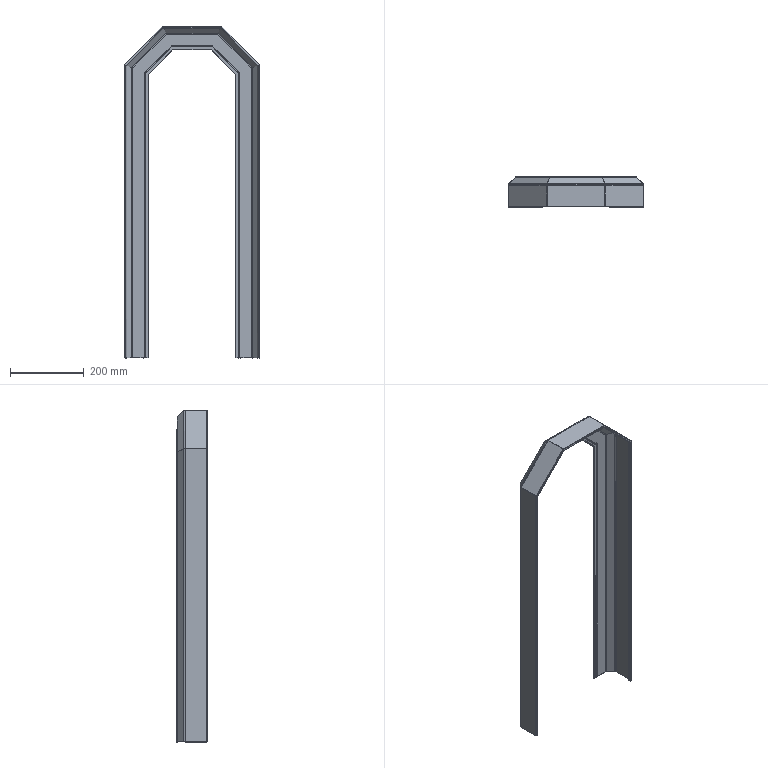Part | STEP file | 51E-01207JG10 | 1 solid | 217 faces | box 367.304 x 82.9 x 899.652 mm | volume 410628 mm3 | cylinder 150 | plane 67 | commonest cylinder face diameters 1 x45 1.8 x30 0.9 x20 0.4 x15 0.6 x10 3 x10